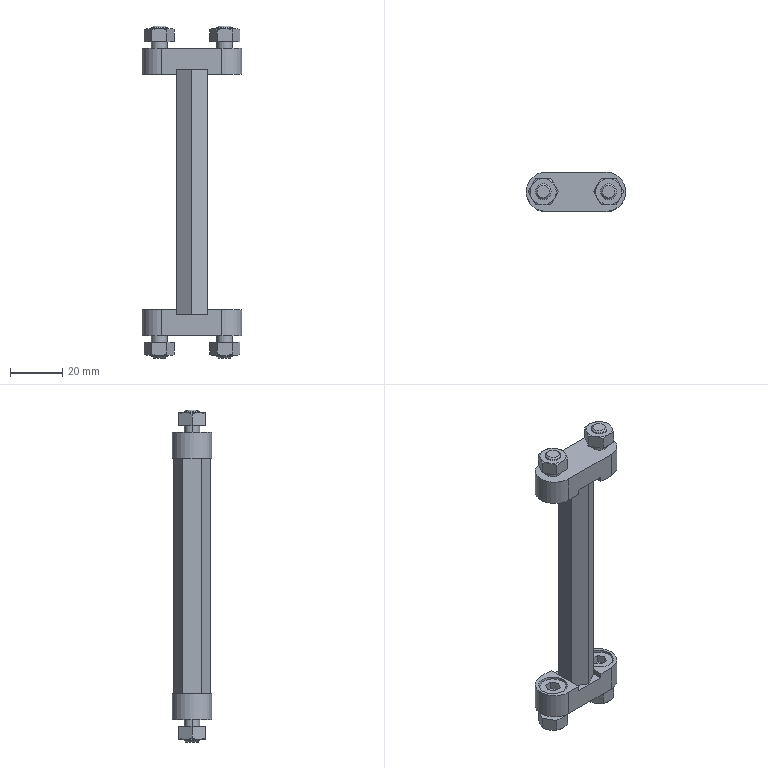Part | STEP file | Guide wheel mechanism revised.sldasm-Part-74 | 1 solid | 194 faces | box 38 x 15 x 127 mm | volume 22589 mm3 | plane 104 | cylinder 46 | cone 44 | commonest cylinder face diameters 6 x16 6.4 x8 10 x8 11 x8 15 x6